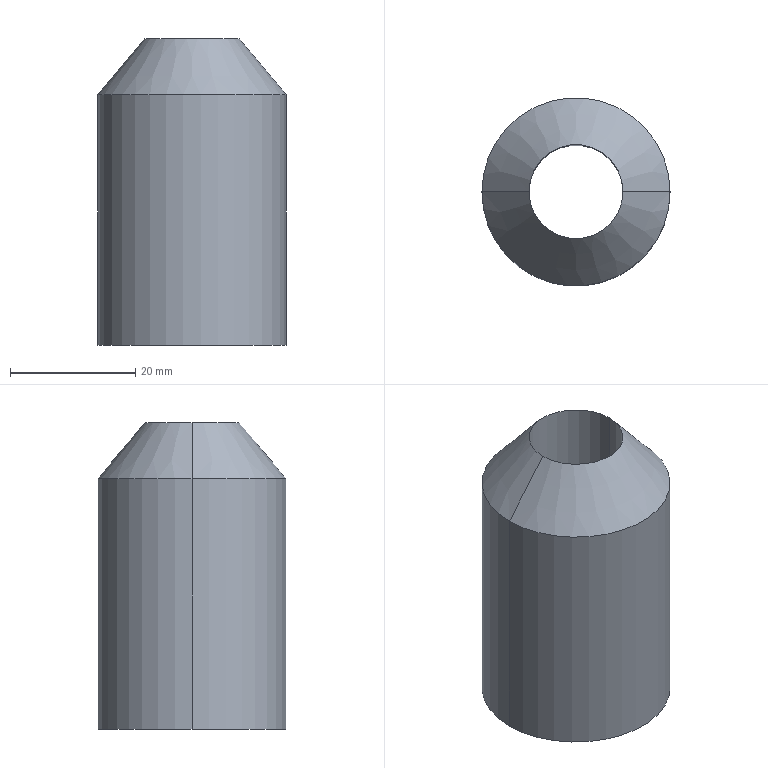Part | SolidWorks | features Chamfer 1, Extrusion 1 | 1 solid | 7 faces | box 30 x 30 x 48.938 mm | volume 23312 mm3 | cylinder 4 | cone 2 | plane 1 | commonest cylinder face diameters 15 x2 30 x2
STEP:
#1=CARTESIAN_POINT('',(7.5,0.,48.938));
#2=VERTEX_POINT('',#1);
#3=CARTESIAN_POINT('',(-7.5,0.,48.938));
#4=VERTEX_POINT('',#3);
#5=CARTESIAN_POINT('',(0.,0.,48.938));
#6=DIRECTION('',(0.,0.,1.));
#7=DIRECTION('',(-1.,0.,0.));
#8=AXIS2_PLACEMENT_3D('',#5,#6,#7);
#9=CIRCLE('',#8,7.5);
#10=EDGE_CURVE('',#2,#4,#9,.T.);
#11=ORIENTED_EDGE('',*,*,#10,.F.);
#12=CARTESIAN_POINT('',(15.,0.,40.));
#13=VERTEX_POINT('',#12);
#14=CARTESIAN_POINT('',(6.609,0.,50.));
#15=DIRECTION('',(0.6428,0.,-0.766));
#16=VECTOR('',#15,1000.);
#17=LINE('',#14,#16);
#18=EDGE_CURVE('',#2,#13,#17,.T.);
#19=ORIENTED_EDGE('',*,*,#18,.T.);
#20=CARTESIAN_POINT('',(-15.,0.,40.));
#21=VERTEX_POINT('',#20);
#22=CARTESIAN_POINT('',(0.,0.,40.));
#23=DIRECTION('',(0.,0.,-1.));
#24=DIRECTION('',(1.,0.,0.));
#25=AXIS2_PLACEMENT_3D('',#22,#23,#24);
#26=CIRCLE('',#25,15.);
#27=EDGE_CURVE('',#21,#13,#26,.T.);
#28=ORIENTED_EDGE('',*,*,#27,.F.);
#29=CARTESIAN_POINT('',(-6.609,0.,50.));
#30=DIRECTION('',(-0.6428,0.,-0.766));
#31=VECTOR('',#30,1000.);
#32=LINE('',#29,#31);
#33=EDGE_CURVE('',#4,#21,#32,.T.);
#34=ORIENTED_EDGE('',*,*,#33,.F.);
#35=EDGE_LOOP('',(#11,#19,#28,#34));
#36=FACE_OUTER_BOUND('',#35,.T.);
#37=CARTESIAN_POINT('',(0.,0.,50.));
#38=DIRECTION('',(0.,0.,-1.));
#39=DIRECTION('',(-1.,0.,0.));
#40=AXIS2_PLACEMENT_3D('',#37,#38,#39);
#41=CONICAL_SURFACE('',#40,6.609,0.6981);
#42=ADVANCED_FACE('',(#36),#41,.T.);
#43=CARTESIAN_POINT('',(0.,0.,48.938));
#44=DIRECTION('',(0.,0.,1.));
#45=DIRECTION('',(-1.,0.,0.));
#46=AXIS2_PLACEMENT_3D('',#43,#44,#45);
#47=CIRCLE('',#46,7.5);
#48=EDGE_CURVE('',#4,#2,#47,.T.);
#49=ORIENTED_EDGE('',*,*,#48,.T.);
#50=CARTESIAN_POINT('',(7.5,0.,0.));
#51=VERTEX_POINT('',#50);
#52=CARTESIAN_POINT('',(7.5,0.,50.));
#53=DIRECTION('',(0.,0.,-1.));
#54=VECTOR('',#53,1000.);
#55=LINE('',#52,#54);
#56=EDGE_CURVE('',#2,#51,#55,.T.);
#57=ORIENTED_EDGE('',*,*,#56,.T.);
#58=CARTESIAN_POINT('',(-7.5,0.,0.));
#59=VERTEX_POINT('',#58);
#60=CARTESIAN_POINT('',(0.,0.,0.));
#61=DIRECTION('',(0.,0.,1.));
#62=DIRECTION('',(1.,0.,0.));
#63=AXIS2_PLACEMENT_3D('',#60,#61,#62);
#64=CIRCLE('',#63,7.5);
#65=EDGE_CURVE('',#59,#51,#64,.T.);
#66=ORIENTED_EDGE('',*,*,#65,.F.);
#67=CARTESIAN_POINT('',(-7.5,0.,50.));
#68=DIRECTION('',(0.,0.,-1.));
#69=VECTOR('',#68,1000.);
#70=LINE('',#67,#69);
#71=EDGE_CURVE('',#4,#59,#70,.T.);
#72=ORIENTED_EDGE('',*,*,#71,.F.);
#73=EDGE_LOOP('',(#49,#57,#66,#72));
#74=FACE_OUTER_BOUND('',#73,.T.);
#75=CARTESIAN_POINT('',(0.,0.,50.));
#76=DIRECTION('',(0.,0.,-1.));
#77=DIRECTION('',(-1.,0.,0.));
#78=AXIS2_PLACEMENT_3D('',#75,#76,#77);
#79=CYLINDRICAL_SURFACE('',#78,7.5);
#80=ADVANCED_FACE('',(#74),#79,.F.);
#81=ORIENTED_EDGE('',*,*,#27,.T.);
#82=CARTESIAN_POINT('',(15.,0.,0.));
#83=VERTEX_POINT('',#82);
#84=CARTESIAN_POINT('',(15.,0.,50.));
#85=DIRECTION('',(0.,0.,-1.));
#86=VECTOR('',#85,1000.);
#87=LINE('',#84,#86);
#88=EDGE_CURVE('',#13,#83,#87,.T.);
#89=ORIENTED_EDGE('',*,*,#88,.T.);
#90=CARTESIAN_POINT('',(-15.,0.,0.));
#91=VERTEX_POINT('',#90);
#92=CARTESIAN_POINT('',(0.,0.,0.));
#93=DIRECTION('',(0.,0.,1.));
#94=DIRECTION('',(1.,0.,0.));
#95=AXIS2_PLACEMENT_3D('',#92,#93,#94);
#96=CIRCLE('',#95,15.);
#97=EDGE_CURVE('',#83,#91,#96,.T.);
#98=ORIENTED_EDGE('',*,*,#97,.T.);
#99=CARTESIAN_POINT('',(-15.,0.,50.));
#100=DIRECTION('',(0.,0.,-1.));
#101=VECTOR('',#100,1000.);
#102=LINE('',#99,#101);
#103=EDGE_CURVE('',#21,#91,#102,.T.);
#104=ORIENTED_EDGE('',*,*,#103,.F.);
#105=EDGE_LOOP('',(#81,#89,#98,#104));
#106=FACE_OUTER_BOUND('',#105,.T.);
#107=CARTESIAN_POINT('',(0.,0.,50.));
#108=DIRECTION('',(0.,0.,-1.));
#109=DIRECTION('',(-1.,0.,0.));
#110=AXIS2_PLACEMENT_3D('',#107,#108,#109);
#111=CYLINDRICAL_SURFACE('',#110,15.);
#112=ADVANCED_FACE('',(#106),#111,.T.);
#113=CARTESIAN_POINT('',(0.,0.,0.));
#114=DIRECTION('',(0.,0.,1.));
#115=DIRECTION('',(1.,0.,0.));
#116=AXIS2_PLACEMENT_3D('',#113,#114,#115);
#117=CIRCLE('',#116,15.);
#118=EDGE_CURVE('',#91,#83,#117,.T.);
#119=ORIENTED_EDGE('',*,*,#118,.F.);
#120=ORIENTED_EDGE('',*,*,#97,.F.);
#121=EDGE_LOOP('',(#119,#120));
#122=FACE_OUTER_BOUND('',#121,.T.);
#123=ORIENTED_EDGE('',*,*,#65,.T.);
#124=CARTESIAN_POINT('',(0.,0.,0.));
#125=DIRECTION('',(0.,0.,1.));
#126=DIRECTION('',(1.,0.,0.));
#127=AXIS2_PLACEMENT_3D('',#124,#125,#126);
#128=CIRCLE('',#127,7.5);
#129=EDGE_CURVE('',#51,#59,#128,.T.);
#130=ORIENTED_EDGE('',*,*,#129,.T.);
#131=EDGE_LOOP('',(#123,#130));
#132=FACE_BOUND('',#131,.T.);
#133=CARTESIAN_POINT('',(0.,0.,0.));
#134=DIRECTION('',(0.,0.,1.));
#135=DIRECTION('',(1.,0.,0.));
#136=AXIS2_PLACEMENT_3D('',#133,#134,#135);
#137=PLANE('',#136);
#138=ADVANCED_FACE('',(#122,#132),#137,.F.);
#139=ORIENTED_EDGE('',*,*,#88,.F.);
#140=CARTESIAN_POINT('',(0.,0.,40.));
#141=DIRECTION('',(0.,0.,-1.));
#142=DIRECTION('',(1.,0.,0.));
#143=AXIS2_PLACEMENT_3D('',#140,#141,#142);
#144=CIRCLE('',#143,15.);
#145=EDGE_CURVE('',#13,#21,#144,.T.);
#146=ORIENTED_EDGE('',*,*,#145,.T.);
#147=ORIENTED_EDGE('',*,*,#103,.T.);
#148=ORIENTED_EDGE('',*,*,#118,.T.);
#149=EDGE_LOOP('',(#139,#146,#147,#148));
#150=FACE_OUTER_BOUND('',#149,.T.);
#151=CARTESIAN_POINT('',(0.,0.,50.));
#152=DIRECTION('',(0.,0.,-1.));
#153=DIRECTION('',(-1.,0.,0.));
#154=AXIS2_PLACEMENT_3D('',#151,#152,#153);
#155=CYLINDRICAL_SURFACE('',#154,15.);
#156=ADVANCED_FACE('',(#150),#155,.T.);
#157=ORIENTED_EDGE('',*,*,#56,.F.);
#158=ORIENTED_EDGE('',*,*,#10,.T.);
#159=ORIENTED_EDGE('',*,*,#71,.T.);
#160=ORIENTED_EDGE('',*,*,#129,.F.);
#161=EDGE_LOOP('',(#157,#158,#159,#160));
#162=FACE_OUTER_BOUND('',#161,.T.);
#163=CARTESIAN_POINT('',(0.,0.,50.));
#164=DIRECTION('',(0.,0.,-1.));
#165=DIRECTION('',(-1.,0.,0.));
#166=AXIS2_PLACEMENT_3D('',#163,#164,#165);
#167=CYLINDRICAL_SURFACE('',#166,7.5);
#168=ADVANCED_FACE('',(#162),#167,.F.);
#169=ORIENTED_EDGE('',*,*,#18,.F.);
#170=ORIENTED_EDGE('',*,*,#48,.F.);
#171=ORIENTED_EDGE('',*,*,#33,.T.);
#172=ORIENTED_EDGE('',*,*,#145,.F.);
#173=EDGE_LOOP('',(#169,#170,#171,#172));
#174=FACE_OUTER_BOUND('',#173,.T.);
#175=CARTESIAN_POINT('',(0.,0.,50.));
#176=DIRECTION('',(0.,0.,-1.));
#177=DIRECTION('',(-1.,0.,0.));
#178=AXIS2_PLACEMENT_3D('',#175,#176,#177);
#179=CONICAL_SURFACE('',#178,6.609,0.6981);
#180=ADVANCED_FACE('',(#174),#179,.T.);
#181=CLOSED_SHELL('',(#42,#80,#112,#138,#156,#168,#180));
#182=MANIFOLD_SOLID_BREP('',#181);
#183=CARTESIAN_POINT('',(0.,0.,0.));
#184=DIRECTION('',(0.,0.,1.));
#185=DIRECTION('',(1.,0.,0.));
#186=AXIS2_PLACEMENT_3D('',#183,#184,#185);
#187=(LENGTH_UNIT()NAMED_UNIT(*)SI_UNIT(.MILLI.,.METRE.));
#188=UNCERTAINTY_MEASURE_WITH_UNIT(LENGTH_MEASURE(0.00001),#187,'','');
#189=(NAMED_UNIT(*)PLANE_ANGLE_UNIT()SI_UNIT($,.RADIAN.));
#190=(NAMED_UNIT(*)SI_UNIT($,.STERADIAN.)SOLID_ANGLE_UNIT());
#191=(GEOMETRIC_REPRESENTATION_CONTEXT(3)GLOBAL_UNCERTAINTY_ASSIGNED_CONTEXT((#188))GLOBAL_UNIT_ASSIGNED_CONTEXT((#187,#189,#190))REPRESENTATION_CONTEXT('',''));
#192=ADVANCED_BREP_SHAPE_REPRESENTATION('',(#182,#186),#191);